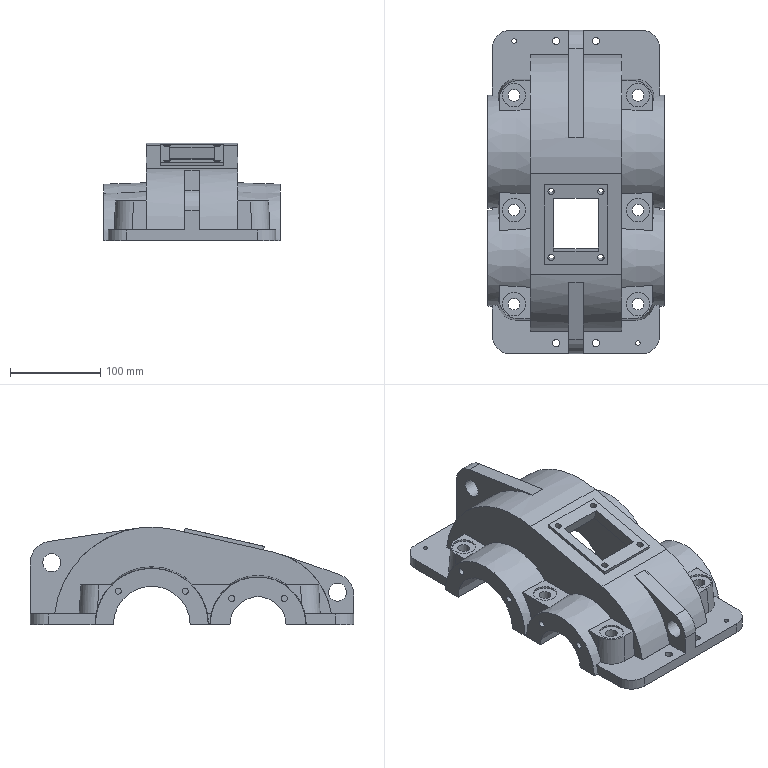Part | NX | features DATUM_CSYS 38, SIMPLE HOLE 38, SKETCH 37, EXTRACT_DATUM_AXIS 32, EXTRACT_FACE 26, HOLE PACKAGE 25, EXTRUDE 21, EXTRACT_DATUM_PLANE 14, Instance Feature 10, DRAFT 8, EXTRACT_STRING 8, BLEND 5, FSET 4, Mirror Feature 4, OFFSET_REGION 3, REPLACE_FACE 3, CPROJ 2, Pattern Feature 2, DATUM_PLANE 1, TRIM BODY 1 | 1 solid | 133 faces | box 195 x 358 x 108 mm | volume 1561648 mm3 | plane 79 | cylinder 50 | cone 4 | commonest cylinder face diameters 7 x12 40 x8 13 x6 26 x6 8 x4 5 x2